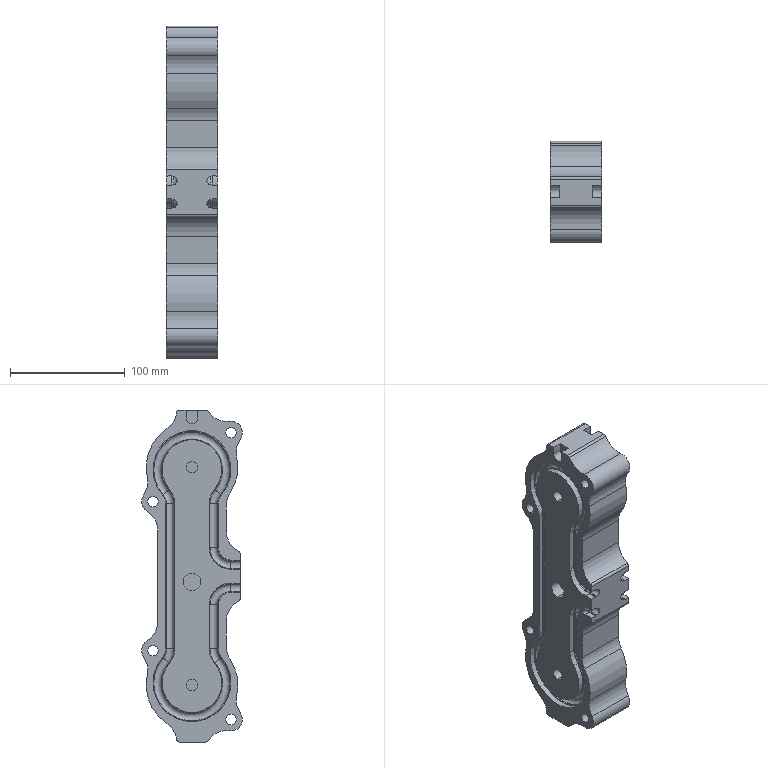Part | STEP file | V802 | 1 solid | 239 faces | box 45 x 88 x 289.568 mm | volume 783132 mm3 | cylinder 110 | plane 69 | cone 44 | torus 16 | commonest cylinder face diameters 6.8 x18 38 x14 23.2 x12 36.8 x12 5 x10 15 x10